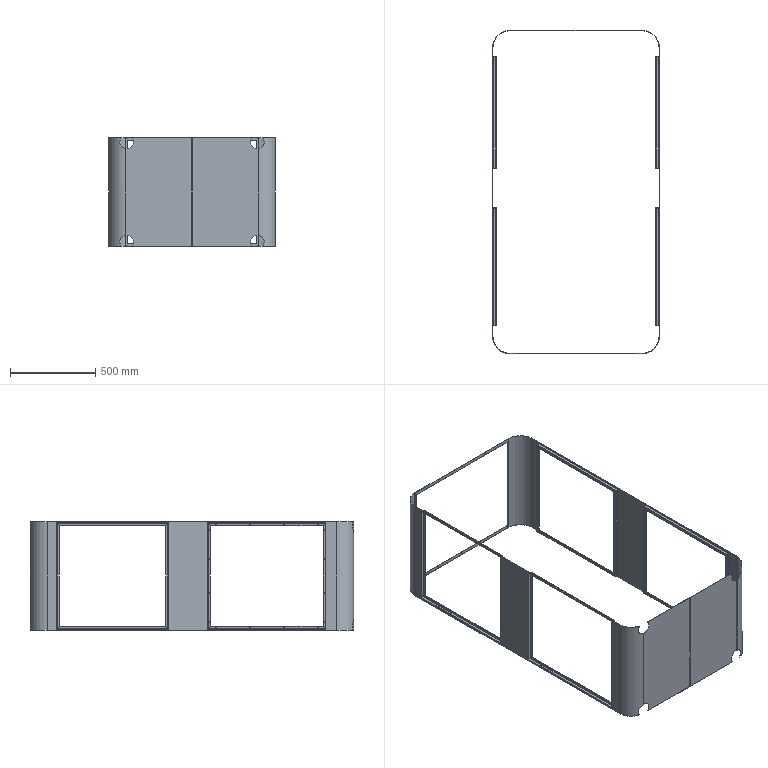Part | STEP file | Split housing part 0101001 | 1 solid | 430 faces | box 980 x 1900 x 640 mm | volume 2630768 mm3 | cylinder 188 | plane 178 | spline 64 | commonest cylinder face diameters 3.5 x64 3 x32 4 x32 6 x32 80 x12 5 x8